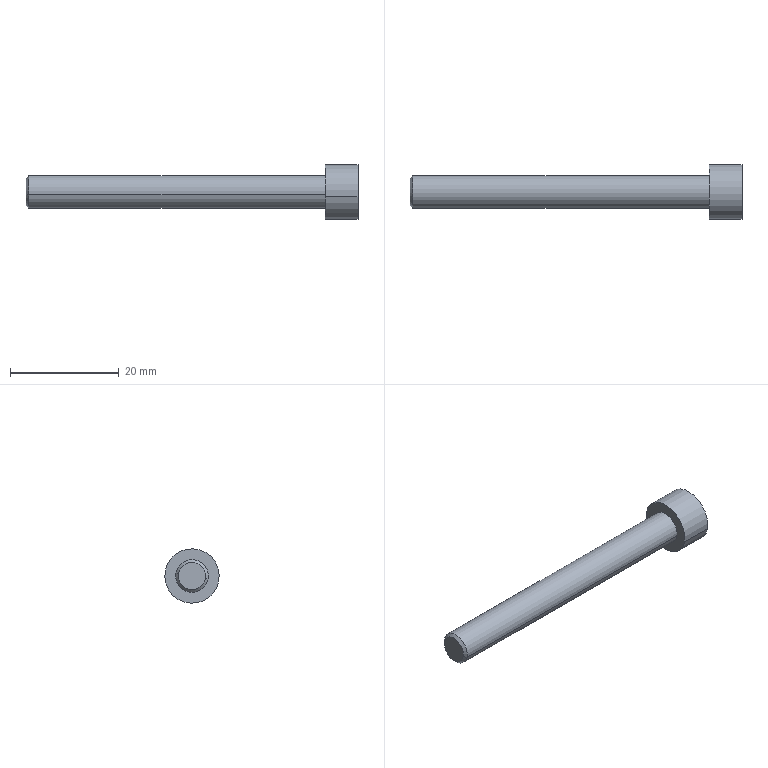Part | SolidWorks | features BaseBody 1 | 1 solid | 16 faces | box 61 x 10 x 10 mm | volume 1959 mm3 | plane 10 | cylinder 4 | cone 2 | commonest cylinder face diameters 6 x2 10 x2
STEP:
#1=CARTESIAN_POINT('',(351.4,87.458,41.455));
#2=VERTEX_POINT('',#1);
#3=CARTESIAN_POINT('',(351.4,82.542,40.545));
#4=VERTEX_POINT('',#3);
#5=CARTESIAN_POINT('',(351.4,85.,41.));
#6=DIRECTION('',(-1.,0.,0.));
#7=DIRECTION('',(0.,0.9833,0.182));
#8=AXIS2_PLACEMENT_3D('',#5,#6,#7);
#9=CIRCLE('',#8,2.5);
#10=EDGE_CURVE('',#2,#4,#9,.T.);
#11=ORIENTED_EDGE('',*,*,#10,.F.);
#12=CARTESIAN_POINT('',(351.9,87.95,41.546));
#13=VERTEX_POINT('',#12);
#14=CARTESIAN_POINT('',(351.4,87.458,41.455));
#15=DIRECTION('',(0.7071,0.6953,0.1287));
#16=VECTOR('',#15,1000.);
#17=LINE('',#14,#16);
#18=EDGE_CURVE('',#2,#13,#17,.T.);
#19=ORIENTED_EDGE('',*,*,#18,.T.);
#20=CARTESIAN_POINT('',(351.9,82.05,40.454));
#21=VERTEX_POINT('',#20);
#22=CARTESIAN_POINT('',(351.9,85.,41.));
#23=DIRECTION('',(1.,0.,0.));
#24=DIRECTION('',(0.,0.9833,0.182));
#25=AXIS2_PLACEMENT_3D('',#22,#23,#24);
#26=CIRCLE('',#25,3.);
#27=EDGE_CURVE('',#21,#13,#26,.T.);
#28=ORIENTED_EDGE('',*,*,#27,.F.);
#29=CARTESIAN_POINT('',(351.4,82.542,40.545));
#30=DIRECTION('',(0.7071,-0.6953,-0.1287));
#31=VECTOR('',#30,1000.);
#32=LINE('',#29,#31);
#33=EDGE_CURVE('',#4,#21,#32,.T.);
#34=ORIENTED_EDGE('',*,*,#33,.F.);
#35=EDGE_LOOP('',(#11,#19,#28,#34));
#36=FACE_OUTER_BOUND('',#35,.T.);
#37=CARTESIAN_POINT('',(351.4,85.,41.));
#38=DIRECTION('',(1.,0.,0.));
#39=DIRECTION('',(0.,-0.9833,-0.182));
#40=AXIS2_PLACEMENT_3D('',#37,#38,#39);
#41=CONICAL_SURFACE('',#40,2.5,0.7854);
#42=ADVANCED_FACE('',(#36),#41,.T.);
#43=ORIENTED_EDGE('',*,*,#27,.T.);
#44=CARTESIAN_POINT('',(406.4,87.95,41.546));
#45=VERTEX_POINT('',#44);
#46=CARTESIAN_POINT('',(351.4,87.95,41.546));
#47=DIRECTION('',(1.,0.,0.));
#48=VECTOR('',#47,1000.);
#49=LINE('',#46,#48);
#50=EDGE_CURVE('',#13,#45,#49,.T.);
#51=ORIENTED_EDGE('',*,*,#50,.T.);
#52=CARTESIAN_POINT('',(406.4,82.05,40.454));
#53=VERTEX_POINT('',#52);
#54=CARTESIAN_POINT('',(406.4,85.,41.));
#55=DIRECTION('',(-1.,0.,0.));
#56=DIRECTION('',(0.,0.9833,0.182));
#57=AXIS2_PLACEMENT_3D('',#54,#55,#56);
#58=CIRCLE('',#57,3.);
#59=EDGE_CURVE('',#45,#53,#58,.T.);
#60=ORIENTED_EDGE('',*,*,#59,.T.);
#61=CARTESIAN_POINT('',(351.4,82.05,40.454));
#62=DIRECTION('',(1.,0.,0.));
#63=VECTOR('',#62,1000.);
#64=LINE('',#61,#63);
#65=EDGE_CURVE('',#21,#53,#64,.T.);
#66=ORIENTED_EDGE('',*,*,#65,.F.);
#67=EDGE_LOOP('',(#43,#51,#60,#66));
#68=FACE_OUTER_BOUND('',#67,.T.);
#69=CARTESIAN_POINT('',(351.4,85.,41.));
#70=DIRECTION('',(1.,0.,0.));
#71=DIRECTION('',(0.,-0.9833,-0.182));
#72=AXIS2_PLACEMENT_3D('',#69,#70,#71);
#73=CYLINDRICAL_SURFACE('',#72,3.);
#74=ADVANCED_FACE('',(#68),#73,.T.);
#75=CARTESIAN_POINT('',(406.4,89.916,41.91));
#76=VERTEX_POINT('',#75);
#77=CARTESIAN_POINT('',(406.4,80.084,40.09));
#78=VERTEX_POINT('',#77);
#79=CARTESIAN_POINT('',(406.4,85.,41.));
#80=DIRECTION('',(-1.,0.,0.));
#81=DIRECTION('',(0.,0.9833,0.182));
#82=AXIS2_PLACEMENT_3D('',#79,#80,#81);
#83=CIRCLE('',#82,5.);
#84=EDGE_CURVE('',#76,#78,#83,.T.);
#85=ORIENTED_EDGE('',*,*,#84,.F.);
#86=CARTESIAN_POINT('',(412.4,89.916,41.91));
#87=VERTEX_POINT('',#86);
#88=CARTESIAN_POINT('',(406.4,89.916,41.91));
#89=DIRECTION('',(1.,0.,0.));
#90=VECTOR('',#89,1000.);
#91=LINE('',#88,#90);
#92=EDGE_CURVE('',#76,#87,#91,.T.);
#93=ORIENTED_EDGE('',*,*,#92,.T.);
#94=CARTESIAN_POINT('',(412.4,80.084,40.09));
#95=VERTEX_POINT('',#94);
#96=CARTESIAN_POINT('',(412.4,85.,41.));
#97=DIRECTION('',(-1.,0.,0.));
#98=DIRECTION('',(0.,0.9833,0.182));
#99=AXIS2_PLACEMENT_3D('',#96,#97,#98);
#100=CIRCLE('',#99,5.);
#101=EDGE_CURVE('',#87,#95,#100,.T.);
#102=ORIENTED_EDGE('',*,*,#101,.T.);
#103=CARTESIAN_POINT('',(406.4,80.084,40.09));
#104=DIRECTION('',(1.,0.,0.));
#105=VECTOR('',#104,1000.);
#106=LINE('',#103,#105);
#107=EDGE_CURVE('',#78,#95,#106,.T.);
#108=ORIENTED_EDGE('',*,*,#107,.F.);
#109=EDGE_LOOP('',(#85,#93,#102,#108));
#110=FACE_OUTER_BOUND('',#109,.T.);
#111=CARTESIAN_POINT('',(406.4,85.,41.));
#112=DIRECTION('',(1.,0.,0.));
#113=DIRECTION('',(0.,-0.9833,-0.182));
#114=AXIS2_PLACEMENT_3D('',#111,#112,#113);
#115=CYLINDRICAL_SURFACE('',#114,5.);
#116=ADVANCED_FACE('',(#110),#115,.T.);
#117=CARTESIAN_POINT('',(406.4,85.,41.));
#118=DIRECTION('',(-1.,0.,0.));
#119=DIRECTION('',(0.,0.9833,0.182));
#120=AXIS2_PLACEMENT_3D('',#117,#118,#119);
#121=CIRCLE('',#120,5.);
#122=EDGE_CURVE('',#78,#76,#121,.T.);
#123=ORIENTED_EDGE('',*,*,#122,.T.);
#124=ORIENTED_EDGE('',*,*,#84,.T.);
#125=EDGE_LOOP('',(#123,#124));
#126=FACE_OUTER_BOUND('',#125,.T.);
#127=CARTESIAN_POINT('',(406.4,85.,41.));
#128=DIRECTION('',(-1.,0.,0.));
#129=DIRECTION('',(0.,0.9833,0.182));
#130=AXIS2_PLACEMENT_3D('',#127,#128,#129);
#131=CIRCLE('',#130,3.);
#132=EDGE_CURVE('',#53,#45,#131,.T.);
#133=ORIENTED_EDGE('',*,*,#132,.F.);
#134=ORIENTED_EDGE('',*,*,#59,.F.);
#135=EDGE_LOOP('',(#133,#134));
#136=FACE_BOUND('',#135,.T.);
#137=CARTESIAN_POINT('',(406.4,85.,41.));
#138=DIRECTION('',(-1.,0.,0.));
#139=DIRECTION('',(0.,0.9833,0.182));
#140=AXIS2_PLACEMENT_3D('',#137,#138,#139);
#141=PLANE('',#140);
#142=ADVANCED_FACE('',(#126,#136),#141,.T.);
#143=ORIENTED_EDGE('',*,*,#92,.F.);
#144=ORIENTED_EDGE('',*,*,#122,.F.);
#145=ORIENTED_EDGE('',*,*,#107,.T.);
#146=CARTESIAN_POINT('',(412.4,85.,41.));
#147=DIRECTION('',(-1.,0.,0.));
#148=DIRECTION('',(0.,0.9833,0.182));
#149=AXIS2_PLACEMENT_3D('',#146,#147,#148);
#150=CIRCLE('',#149,5.);
#151=EDGE_CURVE('',#95,#87,#150,.T.);
#152=ORIENTED_EDGE('',*,*,#151,.T.);
#153=EDGE_LOOP('',(#143,#144,#145,#152));
#154=FACE_OUTER_BOUND('',#153,.T.);
#155=CARTESIAN_POINT('',(406.4,85.,41.));
#156=DIRECTION('',(1.,0.,0.));
#157=DIRECTION('',(0.,-0.9833,-0.182));
#158=AXIS2_PLACEMENT_3D('',#155,#156,#157);
#159=CYLINDRICAL_SURFACE('',#158,5.);
#160=ADVANCED_FACE('',(#154),#159,.T.);
#161=CARTESIAN_POINT('',(412.4,87.721,40.036));
#162=VERTEX_POINT('',#161);
#163=CARTESIAN_POINT('',(412.4,87.196,42.874));
#164=VERTEX_POINT('',#163);
#165=CARTESIAN_POINT('',(412.4,87.721,40.036));
#166=DIRECTION('',(0.,-0.182,0.9833));
#167=VECTOR('',#166,1000.);
#168=LINE('',#165,#167);
#169=EDGE_CURVE('',#162,#164,#168,.T.);
#170=ORIENTED_EDGE('',*,*,#169,.F.);
#171=CARTESIAN_POINT('',(412.4,85.525,38.161));
#172=VERTEX_POINT('',#171);
#173=CARTESIAN_POINT('',(412.4,85.525,38.161));
#174=DIRECTION('',(0.,0.7606,0.6493));
#175=VECTOR('',#174,1000.);
#176=LINE('',#173,#175);
#177=EDGE_CURVE('',#172,#162,#176,.T.);
#178=ORIENTED_EDGE('',*,*,#177,.F.);
#179=CARTESIAN_POINT('',(412.4,82.804,39.126));
#180=VERTEX_POINT('',#179);
#181=CARTESIAN_POINT('',(412.4,85.525,38.161));
#182=DIRECTION('',(0.,0.9426,-0.334));
#183=VECTOR('',#182,1000.);
#184=LINE('',#181,#183);
#185=EDGE_CURVE('',#180,#172,#184,.T.);
#186=ORIENTED_EDGE('',*,*,#185,.F.);
#187=CARTESIAN_POINT('',(412.4,82.279,41.964));
#188=VERTEX_POINT('',#187);
#189=CARTESIAN_POINT('',(412.4,82.804,39.126));
#190=DIRECTION('',(0.,0.182,-0.9833));
#191=VECTOR('',#190,1000.);
#192=LINE('',#189,#191);
#193=EDGE_CURVE('',#188,#180,#192,.T.);
#194=ORIENTED_EDGE('',*,*,#193,.F.);
#195=CARTESIAN_POINT('',(412.4,84.475,43.839));
#196=VERTEX_POINT('',#195);
#197=CARTESIAN_POINT('',(412.4,84.475,43.839));
#198=DIRECTION('',(0.,-0.7606,-0.6493));
#199=VECTOR('',#198,1000.);
#200=LINE('',#197,#199);
#201=EDGE_CURVE('',#196,#188,#200,.T.);
#202=ORIENTED_EDGE('',*,*,#201,.F.);
#203=CARTESIAN_POINT('',(412.4,84.475,43.839));
#204=DIRECTION('',(0.,-0.9426,0.334));
#205=VECTOR('',#204,1000.);
#206=LINE('',#203,#205);
#207=EDGE_CURVE('',#164,#196,#206,.T.);
#208=ORIENTED_EDGE('',*,*,#207,.F.);
#209=EDGE_LOOP('',(#170,#178,#186,#194,#202,#208));
#210=FACE_BOUND('',#209,.T.);
#211=ORIENTED_EDGE('',*,*,#151,.F.);
#212=ORIENTED_EDGE('',*,*,#101,.F.);
#213=EDGE_LOOP('',(#211,#212));
#214=FACE_OUTER_BOUND('',#213,.T.);
#215=CARTESIAN_POINT('',(412.4,85.,41.));
#216=DIRECTION('',(-1.,0.,0.));
#217=DIRECTION('',(0.,0.9833,0.182));
#218=AXIS2_PLACEMENT_3D('',#215,#216,#217);
#219=PLANE('',#218);
#220=ADVANCED_FACE('',(#210,#214),#219,.F.);
#221=ORIENTED_EDGE('',*,*,#50,.F.);
#222=CARTESIAN_POINT('',(351.9,85.,41.));
#223=DIRECTION('',(1.,0.,0.));
#224=DIRECTION('',(0.,0.9833,0.182));
#225=AXIS2_PLACEMENT_3D('',#222,#223,#224);
#226=CIRCLE('',#225,3.);
#227=EDGE_CURVE('',#13,#21,#226,.T.);
#228=ORIENTED_EDGE('',*,*,#227,.T.);
#229=ORIENTED_EDGE('',*,*,#65,.T.);
#230=ORIENTED_EDGE('',*,*,#132,.T.);
#231=EDGE_LOOP('',(#221,#228,#229,#230));
#232=FACE_OUTER_BOUND('',#231,.T.);
#233=CARTESIAN_POINT('',(351.4,85.,41.));
#234=DIRECTION('',(1.,0.,0.));
#235=DIRECTION('',(0.,-0.9833,-0.182));
#236=AXIS2_PLACEMENT_3D('',#233,#234,#235);
#237=CYLINDRICAL_SURFACE('',#236,3.);
#238=ADVANCED_FACE('',(#232),#237,.T.);
#239=CARTESIAN_POINT('',(351.4,85.,41.));
#240=DIRECTION('',(-1.,0.,0.));
#241=DIRECTION('',(0.,0.9833,0.182));
#242=AXIS2_PLACEMENT_3D('',#239,#240,#241);
#243=CIRCLE('',#242,2.5);
#244=EDGE_CURVE('',#4,#2,#243,.T.);
#245=ORIENTED_EDGE('',*,*,#244,.T.);
#246=ORIENTED_EDGE('',*,*,#10,.T.);
#247=EDGE_LOOP('',(#245,#246));
#248=FACE_OUTER_BOUND('',#247,.T.);
#249=CARTESIAN_POINT('',(351.4,85.,41.));
#250=DIRECTION('',(-1.,0.,0.));
#251=DIRECTION('',(0.,0.9833,0.182));
#252=AXIS2_PLACEMENT_3D('',#249,#250,#251);
#253=PLANE('',#252);
#254=ADVANCED_FACE('',(#248),#253,.T.);
#255=ORIENTED_EDGE('',*,*,#177,.T.);
#256=CARTESIAN_POINT('',(409.4,87.721,40.036));
#257=VERTEX_POINT('',#256);
#258=CARTESIAN_POINT('',(409.4,87.721,40.036));
#259=DIRECTION('',(1.,0.,0.));
#260=VECTOR('',#259,1000.);
#261=LINE('',#258,#260);
#262=EDGE_CURVE('',#257,#162,#261,.T.);
#263=ORIENTED_EDGE('',*,*,#262,.F.);
#264=CARTESIAN_POINT('',(409.4,85.525,38.161));
#265=VERTEX_POINT('',#264);
#266=CARTESIAN_POINT('',(409.4,85.525,38.161));
#267=DIRECTION('',(0.,0.7606,0.6493));
#268=VECTOR('',#267,1000.);
#269=LINE('',#266,#268);
#270=EDGE_CURVE('',#265,#257,#269,.T.);
#271=ORIENTED_EDGE('',*,*,#270,.F.);
#272=CARTESIAN_POINT('',(409.4,85.525,38.161));
#273=DIRECTION('',(1.,0.,0.));
#274=VECTOR('',#273,1000.);
#275=LINE('',#272,#274);
#276=EDGE_CURVE('',#265,#172,#275,.T.);
#277=ORIENTED_EDGE('',*,*,#276,.T.);
#278=EDGE_LOOP('',(#255,#263,#271,#277));
#279=FACE_OUTER_BOUND('',#278,.T.);
#280=CARTESIAN_POINT('',(409.4,85.525,38.161));
#281=DIRECTION('',(0.,0.6493,-0.7606));
#282=DIRECTION('',(0.,-0.7606,-0.6493));
#283=AXIS2_PLACEMENT_3D('',#280,#281,#282);
#284=PLANE('',#283);
#285=ADVANCED_FACE('',(#279),#284,.F.);
#286=ORIENTED_EDGE('',*,*,#185,.T.);
#287=ORIENTED_EDGE('',*,*,#276,.F.);
#288=CARTESIAN_POINT('',(409.4,82.804,39.126));
#289=VERTEX_POINT('',#288);
#290=CARTESIAN_POINT('',(409.4,85.525,38.161));
#291=DIRECTION('',(0.,0.9426,-0.334));
#292=VECTOR('',#291,1000.);
#293=LINE('',#290,#292);
#294=EDGE_CURVE('',#289,#265,#293,.T.);
#295=ORIENTED_EDGE('',*,*,#294,.F.);
#296=CARTESIAN_POINT('',(409.4,82.804,39.126));
#297=DIRECTION('',(1.,0.,0.));
#298=VECTOR('',#297,1000.);
#299=LINE('',#296,#298);
#300=EDGE_CURVE('',#289,#180,#299,.T.);
#301=ORIENTED_EDGE('',*,*,#300,.T.);
#302=EDGE_LOOP('',(#286,#287,#295,#301));
#303=FACE_OUTER_BOUND('',#302,.T.);
#304=CARTESIAN_POINT('',(409.4,85.525,38.161));
#305=DIRECTION('',(0.,-0.334,-0.9426));
#306=DIRECTION('',(0.,-0.9426,0.334));
#307=AXIS2_PLACEMENT_3D('',#304,#305,#306);
#308=PLANE('',#307);
#309=ADVANCED_FACE('',(#303),#308,.F.);
#310=ORIENTED_EDGE('',*,*,#193,.T.);
#311=ORIENTED_EDGE('',*,*,#300,.F.);
#312=CARTESIAN_POINT('',(409.4,82.279,41.964));
#313=VERTEX_POINT('',#312);
#314=CARTESIAN_POINT('',(409.4,82.804,39.126));
#315=DIRECTION('',(0.,0.182,-0.9833));
#316=VECTOR('',#315,1000.);
#317=LINE('',#314,#316);
#318=EDGE_CURVE('',#313,#289,#317,.T.);
#319=ORIENTED_EDGE('',*,*,#318,.F.);
#320=CARTESIAN_POINT('',(409.4,82.279,41.964));
#321=DIRECTION('',(1.,0.,0.));
#322=VECTOR('',#321,1000.);
#323=LINE('',#320,#322);
#324=EDGE_CURVE('',#313,#188,#323,.T.);
#325=ORIENTED_EDGE('',*,*,#324,.T.);
#326=EDGE_LOOP('',(#310,#311,#319,#325));
#327=FACE_OUTER_BOUND('',#326,.T.);
#328=CARTESIAN_POINT('',(409.4,82.804,39.126));
#329=DIRECTION('',(0.,-0.9833,-0.182));
#330=DIRECTION('',(-1.,0.,0.));
#331=AXIS2_PLACEMENT_3D('',#328,#329,#330);
#332=PLANE('',#331);
#333=ADVANCED_FACE('',(#327),#332,.F.);
#334=ORIENTED_EDGE('',*,*,#201,.T.);
#335=ORIENTED_EDGE('',*,*,#324,.F.);
#336=CARTESIAN_POINT('',(409.4,84.475,43.839));
#337=VERTEX_POINT('',#336);
#338=CARTESIAN_POINT('',(409.4,84.475,43.839));
#339=DIRECTION('',(0.,-0.7606,-0.6493));
#340=VECTOR('',#339,1000.);
#341=LINE('',#338,#340);
#342=EDGE_CURVE('',#337,#313,#341,.T.);
#343=ORIENTED_EDGE('',*,*,#342,.F.);
#344=CARTESIAN_POINT('',(409.4,84.475,43.839));
#345=DIRECTION('',(1.,0.,0.));
#346=VECTOR('',#345,1000.);
#347=LINE('',#344,#346);
#348=EDGE_CURVE('',#337,#196,#347,.T.);
#349=ORIENTED_EDGE('',*,*,#348,.T.);
#350=EDGE_LOOP('',(#334,#335,#343,#349));
#351=FACE_OUTER_BOUND('',#350,.T.);
#352=CARTESIAN_POINT('',(409.4,84.475,43.839));
#353=DIRECTION('',(0.,-0.6493,0.7606));
#354=DIRECTION('',(0.,0.7606,0.6493));
#355=AXIS2_PLACEMENT_3D('',#352,#353,#354);
#356=PLANE('',#355);
#357=ADVANCED_FACE('',(#351),#356,.F.);
#358=ORIENTED_EDGE('',*,*,#207,.T.);
#359=ORIENTED_EDGE('',*,*,#348,.F.);
#360=CARTESIAN_POINT('',(409.4,87.196,42.874));
#361=VERTEX_POINT('',#360);
#362=CARTESIAN_POINT('',(409.4,84.475,43.839));
#363=DIRECTION('',(0.,-0.9426,0.334));
#364=VECTOR('',#363,1000.);
#365=LINE('',#362,#364);
#366=EDGE_CURVE('',#361,#337,#365,.T.);
#367=ORIENTED_EDGE('',*,*,#366,.F.);
#368=CARTESIAN_POINT('',(409.4,87.196,42.874));
#369=DIRECTION('',(1.,0.,0.));
#370=VECTOR('',#369,1000.);
#371=LINE('',#368,#370);
#372=EDGE_CURVE('',#361,#164,#371,.T.);
#373=ORIENTED_EDGE('',*,*,#372,.T.);
#374=EDGE_LOOP('',(#358,#359,#367,#373));
#375=FACE_OUTER_BOUND('',#374,.T.);
#376=CARTESIAN_POINT('',(409.4,84.475,43.839));
#377=DIRECTION('',(0.,0.334,0.9426));
#378=DIRECTION('',(0.,0.9426,-0.334));
#379=AXIS2_PLACEMENT_3D('',#376,#377,#378);
#380=PLANE('',#379);
#381=ADVANCED_FACE('',(#375),#380,.F.);
#382=ORIENTED_EDGE('',*,*,#169,.T.);
#383=ORIENTED_EDGE('',*,*,#372,.F.);
#384=CARTESIAN_POINT('',(409.4,87.721,40.036));
#385=DIRECTION('',(0.,-0.182,0.9833));
#386=VECTOR('',#385,1000.);
#387=LINE('',#384,#386);
#388=EDGE_CURVE('',#257,#361,#387,.T.);
#389=ORIENTED_EDGE('',*,*,#388,.F.);
#390=ORIENTED_EDGE('',*,*,#262,.T.);
#391=EDGE_LOOP('',(#382,#383,#389,#390));
#392=FACE_OUTER_BOUND('',#391,.T.);
#393=CARTESIAN_POINT('',(409.4,87.721,40.036));
#394=DIRECTION('',(0.,0.9833,0.182));
#395=DIRECTION('',(1.,0.,0.));
#396=AXIS2_PLACEMENT_3D('',#393,#394,#395);
#397=PLANE('',#396);
#398=ADVANCED_FACE('',(#392),#397,.F.);
#399=ORIENTED_EDGE('',*,*,#270,.T.);
#400=ORIENTED_EDGE('',*,*,#388,.T.);
#401=ORIENTED_EDGE('',*,*,#366,.T.);
#402=ORIENTED_EDGE('',*,*,#342,.T.);
#403=ORIENTED_EDGE('',*,*,#318,.T.);
#404=ORIENTED_EDGE('',*,*,#294,.T.);
#405=EDGE_LOOP('',(#399,#400,#401,#402,#403,#404));
#406=FACE_OUTER_BOUND('',#405,.T.);
#407=CARTESIAN_POINT('',(409.4,85.525,38.161));
#408=DIRECTION('',(1.,0.,0.));
#409=DIRECTION('',(0.,-0.9833,-0.182));
#410=AXIS2_PLACEMENT_3D('',#407,#408,#409);
#411=PLANE('',#410);
#412=ADVANCED_FACE('',(#406),#411,.T.);
#413=ORIENTED_EDGE('',*,*,#18,.F.);
#414=ORIENTED_EDGE('',*,*,#244,.F.);
#415=ORIENTED_EDGE('',*,*,#33,.T.);
#416=ORIENTED_EDGE('',*,*,#227,.F.);
#417=EDGE_LOOP('',(#413,#414,#415,#416));
#418=FACE_OUTER_BOUND('',#417,.T.);
#419=CARTESIAN_POINT('',(351.4,85.,41.));
#420=DIRECTION('',(1.,0.,0.));
#421=DIRECTION('',(0.,-0.9833,-0.182));
#422=AXIS2_PLACEMENT_3D('',#419,#420,#421);
#423=CONICAL_SURFACE('',#422,2.5,0.7854);
#424=ADVANCED_FACE('',(#418),#423,.T.);
#425=CLOSED_SHELL('',(#42,#74,#116,#142,#160,#220,#238,#254,#285,#309,#333,#357,#381,#398,#412,#424));
#426=MANIFOLD_SOLID_BREP('',#425);
#427=CARTESIAN_POINT('',(0.,0.,0.));
#428=DIRECTION('',(0.,0.,1.));
#429=DIRECTION('',(1.,0.,0.));
#430=AXIS2_PLACEMENT_3D('',#427,#428,#429);
#431=(LENGTH_UNIT()NAMED_UNIT(*)SI_UNIT(.MILLI.,.METRE.));
#432=UNCERTAINTY_MEASURE_WITH_UNIT(LENGTH_MEASURE(0.00001),#431,'','');
#433=(NAMED_UNIT(*)PLANE_ANGLE_UNIT()SI_UNIT($,.RADIAN.));
#434=(NAMED_UNIT(*)SI_UNIT($,.STERADIAN.)SOLID_ANGLE_UNIT());
#435=(GEOMETRIC_REPRESENTATION_CONTEXT(3)GLOBAL_UNCERTAINTY_ASSIGNED_CONTEXT((#432))GLOBAL_UNIT_ASSIGNED_CONTEXT((#431,#433,#434))REPRESENTATION_CONTEXT('',''));
#436=ADVANCED_BREP_SHAPE_REPRESENTATION('',(#426,#430),#435);